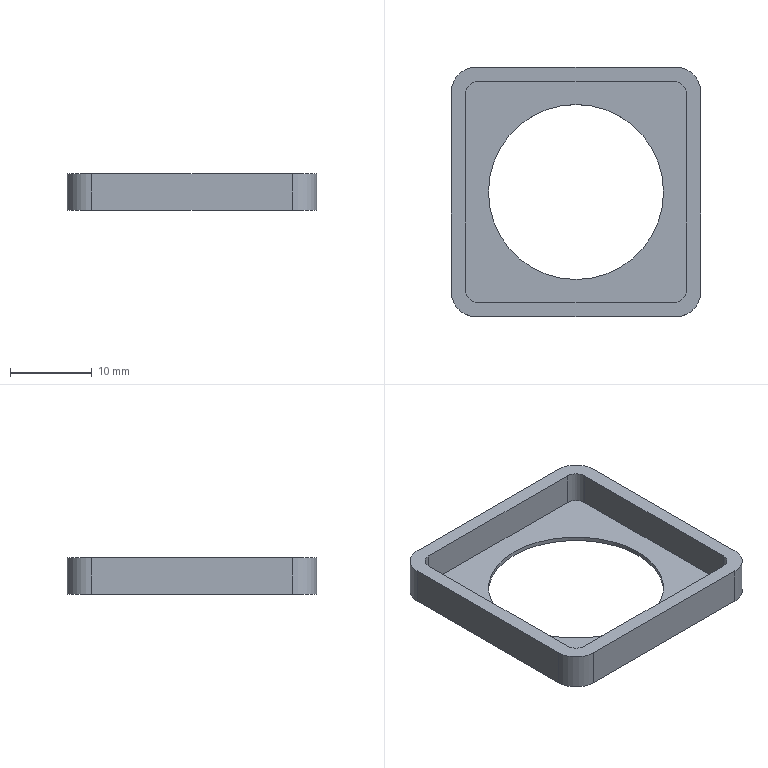Part | STEP file | 1 solid | 21 faces | box 30.5 x 30.5 x 4.5 mm | volume 1063 mm3 | plane 11 | cylinder 10 | commonest cylinder face diameters 3 x4 6 x4 21.4 x2
STEP:
#1=CARTESIAN_POINT('',(10.7,0.,0.));
#2=VERTEX_POINT('',#1);
#3=CARTESIAN_POINT('',(-10.7,0.,0.));
#4=VERTEX_POINT('',#3);
#5=CARTESIAN_POINT('',(0.,0.,0.));
#6=DIRECTION('',(0.,0.,-1.));
#7=DIRECTION('',(-1.,0.,0.));
#8=AXIS2_PLACEMENT_3D('',#5,#6,#7);
#9=CIRCLE('',#8,10.7);
#10=EDGE_CURVE('',#2,#4,#9,.T.);
#11=ORIENTED_EDGE('',*,*,#10,.T.);
#12=CARTESIAN_POINT('',(-10.7,0.,0.5));
#13=VERTEX_POINT('',#12);
#14=CARTESIAN_POINT('',(-10.7,0.,-3.4));
#15=DIRECTION('',(0.,0.,1.));
#16=VECTOR('',#15,1000.);
#17=LINE('',#14,#16);
#18=EDGE_CURVE('',#4,#13,#17,.T.);
#19=ORIENTED_EDGE('',*,*,#18,.T.);
#20=CARTESIAN_POINT('',(10.7,0.,0.5));
#21=VERTEX_POINT('',#20);
#22=CARTESIAN_POINT('',(0.,0.,0.5));
#23=DIRECTION('',(0.,0.,1.));
#24=DIRECTION('',(1.,0.,0.));
#25=AXIS2_PLACEMENT_3D('',#22,#23,#24);
#26=CIRCLE('',#25,10.7);
#27=EDGE_CURVE('',#13,#21,#26,.T.);
#28=ORIENTED_EDGE('',*,*,#27,.T.);
#29=CARTESIAN_POINT('',(10.7,0.,-3.4));
#30=DIRECTION('',(0.,0.,1.));
#31=VECTOR('',#30,1000.);
#32=LINE('',#29,#31);
#33=EDGE_CURVE('',#2,#21,#32,.T.);
#34=ORIENTED_EDGE('',*,*,#33,.F.);
#35=EDGE_LOOP('',(#11,#19,#28,#34));
#36=FACE_OUTER_BOUND('',#35,.T.);
#37=CARTESIAN_POINT('',(0.,0.,-3.4));
#38=DIRECTION('',(0.,0.,1.));
#39=DIRECTION('',(1.,0.,0.));
#40=AXIS2_PLACEMENT_3D('',#37,#38,#39);
#41=CYLINDRICAL_SURFACE('',#40,10.7);
#42=ADVANCED_FACE('',(#36),#41,.F.);
#43=CARTESIAN_POINT('',(-15.25,-12.25,0.));
#44=VERTEX_POINT('',#43);
#45=CARTESIAN_POINT('',(-12.25,-15.25,0.));
#46=VERTEX_POINT('',#45);
#47=CARTESIAN_POINT('',(-12.25,-12.25,0.));
#48=DIRECTION('',(0.,0.,1.));
#49=DIRECTION('',(-1.,0.,0.));
#50=AXIS2_PLACEMENT_3D('',#47,#48,#49);
#51=CIRCLE('',#50,3.);
#52=EDGE_CURVE('',#44,#46,#51,.T.);
#53=ORIENTED_EDGE('',*,*,#52,.T.);
#54=CARTESIAN_POINT('',(-12.25,-15.25,4.5));
#55=VERTEX_POINT('',#54);
#56=CARTESIAN_POINT('',(-12.25,-15.25,4.5));
#57=DIRECTION('',(0.,0.,-1.));
#58=VECTOR('',#57,1000.);
#59=LINE('',#56,#58);
#60=EDGE_CURVE('',#55,#46,#59,.T.);
#61=ORIENTED_EDGE('',*,*,#60,.F.);
#62=CARTESIAN_POINT('',(-15.25,-12.25,4.5));
#63=VERTEX_POINT('',#62);
#64=CARTESIAN_POINT('',(-12.25,-12.25,4.5));
#65=DIRECTION('',(0.,0.,1.));
#66=DIRECTION('',(-1.,0.,0.));
#67=AXIS2_PLACEMENT_3D('',#64,#65,#66);
#68=CIRCLE('',#67,3.);
#69=EDGE_CURVE('',#63,#55,#68,.T.);
#70=ORIENTED_EDGE('',*,*,#69,.F.);
#71=CARTESIAN_POINT('',(-15.25,-12.25,4.5));
#72=DIRECTION('',(0.,0.,-1.));
#73=VECTOR('',#72,1000.);
#74=LINE('',#71,#73);
#75=EDGE_CURVE('',#63,#44,#74,.T.);
#76=ORIENTED_EDGE('',*,*,#75,.T.);
#77=EDGE_LOOP('',(#53,#61,#70,#76));
#78=FACE_OUTER_BOUND('',#77,.T.);
#79=CARTESIAN_POINT('',(-12.25,-12.25,4.5));
#80=DIRECTION('',(0.,0.,-1.));
#81=DIRECTION('',(-1.,0.,0.));
#82=AXIS2_PLACEMENT_3D('',#79,#80,#81);
#83=CYLINDRICAL_SURFACE('',#82,3.);
#84=ADVANCED_FACE('',(#78),#83,.T.);
#85=CARTESIAN_POINT('',(12.25,-15.25,0.));
#86=VERTEX_POINT('',#85);
#87=CARTESIAN_POINT('',(-12.25,-15.25,0.));
#88=DIRECTION('',(1.,0.,0.));
#89=VECTOR('',#88,1000.);
#90=LINE('',#87,#89);
#91=EDGE_CURVE('',#46,#86,#90,.T.);
#92=ORIENTED_EDGE('',*,*,#91,.T.);
#93=CARTESIAN_POINT('',(12.25,-15.25,4.5));
#94=VERTEX_POINT('',#93);
#95=CARTESIAN_POINT('',(12.25,-15.25,4.5));
#96=DIRECTION('',(0.,0.,-1.));
#97=VECTOR('',#96,1000.);
#98=LINE('',#95,#97);
#99=EDGE_CURVE('',#94,#86,#98,.T.);
#100=ORIENTED_EDGE('',*,*,#99,.F.);
#101=CARTESIAN_POINT('',(-12.25,-15.25,4.5));
#102=DIRECTION('',(1.,0.,0.));
#103=VECTOR('',#102,1000.);
#104=LINE('',#101,#103);
#105=EDGE_CURVE('',#55,#94,#104,.T.);
#106=ORIENTED_EDGE('',*,*,#105,.F.);
#107=ORIENTED_EDGE('',*,*,#60,.T.);
#108=EDGE_LOOP('',(#92,#100,#106,#107));
#109=FACE_OUTER_BOUND('',#108,.T.);
#110=CARTESIAN_POINT('',(-12.25,-15.25,4.5));
#111=DIRECTION('',(0.,1.,0.));
#112=DIRECTION('',(1.,0.,0.));
#113=AXIS2_PLACEMENT_3D('',#110,#111,#112);
#114=PLANE('',#113);
#115=ADVANCED_FACE('',(#109),#114,.F.);
#116=CARTESIAN_POINT('',(15.25,-12.25,0.));
#117=VERTEX_POINT('',#116);
#118=CARTESIAN_POINT('',(12.25,-12.25,0.));
#119=DIRECTION('',(0.,0.,1.));
#120=DIRECTION('',(1.,0.,0.));
#121=AXIS2_PLACEMENT_3D('',#118,#119,#120);
#122=CIRCLE('',#121,3.);
#123=EDGE_CURVE('',#86,#117,#122,.T.);
#124=ORIENTED_EDGE('',*,*,#123,.T.);
#125=CARTESIAN_POINT('',(15.25,-12.25,4.5));
#126=VERTEX_POINT('',#125);
#127=CARTESIAN_POINT('',(15.25,-12.25,4.5));
#128=DIRECTION('',(0.,0.,-1.));
#129=VECTOR('',#128,1000.);
#130=LINE('',#127,#129);
#131=EDGE_CURVE('',#126,#117,#130,.T.);
#132=ORIENTED_EDGE('',*,*,#131,.F.);
#133=CARTESIAN_POINT('',(12.25,-12.25,4.5));
#134=DIRECTION('',(0.,0.,1.));
#135=DIRECTION('',(1.,0.,0.));
#136=AXIS2_PLACEMENT_3D('',#133,#134,#135);
#137=CIRCLE('',#136,3.);
#138=EDGE_CURVE('',#94,#126,#137,.T.);
#139=ORIENTED_EDGE('',*,*,#138,.F.);
#140=ORIENTED_EDGE('',*,*,#99,.T.);
#141=EDGE_LOOP('',(#124,#132,#139,#140));
#142=FACE_OUTER_BOUND('',#141,.T.);
#143=CARTESIAN_POINT('',(12.25,-12.25,4.5));
#144=DIRECTION('',(0.,0.,-1.));
#145=DIRECTION('',(-1.,0.,0.));
#146=AXIS2_PLACEMENT_3D('',#143,#144,#145);
#147=CYLINDRICAL_SURFACE('',#146,3.);
#148=ADVANCED_FACE('',(#142),#147,.T.);
#149=CARTESIAN_POINT('',(15.25,12.25,0.));
#150=VERTEX_POINT('',#149);
#151=CARTESIAN_POINT('',(15.25,-12.25,0.));
#152=DIRECTION('',(0.,1.,0.));
#153=VECTOR('',#152,1000.);
#154=LINE('',#151,#153);
#155=EDGE_CURVE('',#117,#150,#154,.T.);
#156=ORIENTED_EDGE('',*,*,#155,.T.);
#157=CARTESIAN_POINT('',(15.25,12.25,4.5));
#158=VERTEX_POINT('',#157);
#159=CARTESIAN_POINT('',(15.25,12.25,4.5));
#160=DIRECTION('',(0.,0.,-1.));
#161=VECTOR('',#160,1000.);
#162=LINE('',#159,#161);
#163=EDGE_CURVE('',#158,#150,#162,.T.);
#164=ORIENTED_EDGE('',*,*,#163,.F.);
#165=CARTESIAN_POINT('',(15.25,-12.25,4.5));
#166=DIRECTION('',(0.,1.,0.));
#167=VECTOR('',#166,1000.);
#168=LINE('',#165,#167);
#169=EDGE_CURVE('',#126,#158,#168,.T.);
#170=ORIENTED_EDGE('',*,*,#169,.F.);
#171=ORIENTED_EDGE('',*,*,#131,.T.);
#172=EDGE_LOOP('',(#156,#164,#170,#171));
#173=FACE_OUTER_BOUND('',#172,.T.);
#174=CARTESIAN_POINT('',(15.25,-12.25,4.5));
#175=DIRECTION('',(-1.,0.,0.));
#176=DIRECTION('',(0.,0.,1.));
#177=AXIS2_PLACEMENT_3D('',#174,#175,#176);
#178=PLANE('',#177);
#179=ADVANCED_FACE('',(#173),#178,.F.);
#180=CARTESIAN_POINT('',(12.25,15.25,0.));
#181=VERTEX_POINT('',#180);
#182=CARTESIAN_POINT('',(12.25,12.25,0.));
#183=DIRECTION('',(0.,0.,1.));
#184=DIRECTION('',(-1.,0.,0.));
#185=AXIS2_PLACEMENT_3D('',#182,#183,#184);
#186=CIRCLE('',#185,3.);
#187=EDGE_CURVE('',#150,#181,#186,.T.);
#188=ORIENTED_EDGE('',*,*,#187,.T.);
#189=CARTESIAN_POINT('',(12.25,15.25,4.5));
#190=VERTEX_POINT('',#189);
#191=CARTESIAN_POINT('',(12.25,15.25,4.5));
#192=DIRECTION('',(0.,0.,-1.));
#193=VECTOR('',#192,1000.);
#194=LINE('',#191,#193);
#195=EDGE_CURVE('',#190,#181,#194,.T.);
#196=ORIENTED_EDGE('',*,*,#195,.F.);
#197=CARTESIAN_POINT('',(12.25,12.25,4.5));
#198=DIRECTION('',(0.,0.,1.));
#199=DIRECTION('',(-1.,0.,0.));
#200=AXIS2_PLACEMENT_3D('',#197,#198,#199);
#201=CIRCLE('',#200,3.);
#202=EDGE_CURVE('',#158,#190,#201,.T.);
#203=ORIENTED_EDGE('',*,*,#202,.F.);
#204=ORIENTED_EDGE('',*,*,#163,.T.);
#205=EDGE_LOOP('',(#188,#196,#203,#204));
#206=FACE_OUTER_BOUND('',#205,.T.);
#207=CARTESIAN_POINT('',(12.25,12.25,4.5));
#208=DIRECTION('',(0.,0.,-1.));
#209=DIRECTION('',(-1.,0.,0.));
#210=AXIS2_PLACEMENT_3D('',#207,#208,#209);
#211=CYLINDRICAL_SURFACE('',#210,3.);
#212=ADVANCED_FACE('',(#206),#211,.T.);
#213=CARTESIAN_POINT('',(-12.25,15.25,0.));
#214=VERTEX_POINT('',#213);
#215=CARTESIAN_POINT('',(-12.25,15.25,0.));
#216=DIRECTION('',(-1.,0.,0.));
#217=VECTOR('',#216,1000.);
#218=LINE('',#215,#217);
#219=EDGE_CURVE('',#181,#214,#218,.T.);
#220=ORIENTED_EDGE('',*,*,#219,.T.);
#221=CARTESIAN_POINT('',(-12.25,15.25,4.5));
#222=VERTEX_POINT('',#221);
#223=CARTESIAN_POINT('',(-12.25,15.25,4.5));
#224=DIRECTION('',(0.,0.,-1.));
#225=VECTOR('',#224,1000.);
#226=LINE('',#223,#225);
#227=EDGE_CURVE('',#222,#214,#226,.T.);
#228=ORIENTED_EDGE('',*,*,#227,.F.);
#229=CARTESIAN_POINT('',(-12.25,15.25,4.5));
#230=DIRECTION('',(-1.,0.,0.));
#231=VECTOR('',#230,1000.);
#232=LINE('',#229,#231);
#233=EDGE_CURVE('',#190,#222,#232,.T.);
#234=ORIENTED_EDGE('',*,*,#233,.F.);
#235=ORIENTED_EDGE('',*,*,#195,.T.);
#236=EDGE_LOOP('',(#220,#228,#234,#235));
#237=FACE_OUTER_BOUND('',#236,.T.);
#238=CARTESIAN_POINT('',(-12.25,15.25,4.5));
#239=DIRECTION('',(0.,-1.,0.));
#240=DIRECTION('',(0.,0.,-1.));
#241=AXIS2_PLACEMENT_3D('',#238,#239,#240);
#242=PLANE('',#241);
#243=ADVANCED_FACE('',(#237),#242,.F.);
#244=CARTESIAN_POINT('',(-15.25,12.25,0.));
#245=VERTEX_POINT('',#244);
#246=CARTESIAN_POINT('',(-12.25,12.25,0.));
#247=DIRECTION('',(0.,0.,1.));
#248=DIRECTION('',(-1.,0.,0.));
#249=AXIS2_PLACEMENT_3D('',#246,#247,#248);
#250=CIRCLE('',#249,3.);
#251=EDGE_CURVE('',#214,#245,#250,.T.);
#252=ORIENTED_EDGE('',*,*,#251,.T.);
#253=CARTESIAN_POINT('',(-15.25,12.25,4.5));
#254=VERTEX_POINT('',#253);
#255=CARTESIAN_POINT('',(-15.25,12.25,4.5));
#256=DIRECTION('',(0.,0.,-1.));
#257=VECTOR('',#256,1000.);
#258=LINE('',#255,#257);
#259=EDGE_CURVE('',#254,#245,#258,.T.);
#260=ORIENTED_EDGE('',*,*,#259,.F.);
#261=CARTESIAN_POINT('',(-12.25,12.25,4.5));
#262=DIRECTION('',(0.,0.,1.));
#263=DIRECTION('',(-1.,0.,0.));
#264=AXIS2_PLACEMENT_3D('',#261,#262,#263);
#265=CIRCLE('',#264,3.);
#266=EDGE_CURVE('',#222,#254,#265,.T.);
#267=ORIENTED_EDGE('',*,*,#266,.F.);
#268=ORIENTED_EDGE('',*,*,#227,.T.);
#269=EDGE_LOOP('',(#252,#260,#267,#268));
#270=FACE_OUTER_BOUND('',#269,.T.);
#271=CARTESIAN_POINT('',(-12.25,12.25,4.5));
#272=DIRECTION('',(0.,0.,-1.));
#273=DIRECTION('',(-1.,0.,0.));
#274=AXIS2_PLACEMENT_3D('',#271,#272,#273);
#275=CYLINDRICAL_SURFACE('',#274,3.);
#276=ADVANCED_FACE('',(#270),#275,.T.);
#277=CARTESIAN_POINT('',(-15.25,-12.25,0.));
#278=DIRECTION('',(0.,-1.,0.));
#279=VECTOR('',#278,1000.);
#280=LINE('',#277,#279);
#281=EDGE_CURVE('',#245,#44,#280,.T.);
#282=ORIENTED_EDGE('',*,*,#281,.T.);
#283=ORIENTED_EDGE('',*,*,#75,.F.);
#284=CARTESIAN_POINT('',(-15.25,-12.25,4.5));
#285=DIRECTION('',(0.,-1.,0.));
#286=VECTOR('',#285,1000.);
#287=LINE('',#284,#286);
#288=EDGE_CURVE('',#254,#63,#287,.T.);
#289=ORIENTED_EDGE('',*,*,#288,.F.);
#290=ORIENTED_EDGE('',*,*,#259,.T.);
#291=EDGE_LOOP('',(#282,#283,#289,#290));
#292=FACE_OUTER_BOUND('',#291,.T.);
#293=CARTESIAN_POINT('',(-15.25,-12.25,4.5));
#294=DIRECTION('',(1.,0.,0.));
#295=DIRECTION('',(0.,1.,0.));
#296=AXIS2_PLACEMENT_3D('',#293,#294,#295);
#297=PLANE('',#296);
#298=ADVANCED_FACE('',(#292),#297,.F.);
#299=ORIENTED_EDGE('',*,*,#69,.T.);
#300=ORIENTED_EDGE('',*,*,#105,.T.);
#301=ORIENTED_EDGE('',*,*,#138,.T.);
#302=ORIENTED_EDGE('',*,*,#169,.T.);
#303=ORIENTED_EDGE('',*,*,#202,.T.);
#304=ORIENTED_EDGE('',*,*,#233,.T.);
#305=ORIENTED_EDGE('',*,*,#266,.T.);
#306=ORIENTED_EDGE('',*,*,#288,.T.);
#307=EDGE_LOOP('',(#299,#300,#301,#302,#303,#304,#305,#306));
#308=FACE_OUTER_BOUND('',#307,.T.);
#309=CARTESIAN_POINT('',(-12.,-13.5,4.5));
#310=VERTEX_POINT('',#309);
#311=CARTESIAN_POINT('',(12.,-13.5,4.5));
#312=VERTEX_POINT('',#311);
#313=CARTESIAN_POINT('',(-12.,-13.5,4.5));
#314=DIRECTION('',(1.,0.,0.));
#315=VECTOR('',#314,1000.);
#316=LINE('',#313,#315);
#317=EDGE_CURVE('',#310,#312,#316,.T.);
#318=ORIENTED_EDGE('',*,*,#317,.F.);
#319=CARTESIAN_POINT('',(-13.5,-12.,4.5));
#320=VERTEX_POINT('',#319);
#321=CARTESIAN_POINT('',(-12.,-12.,4.5));
#322=DIRECTION('',(0.,0.,1.));
#323=DIRECTION('',(-1.,0.,0.));
#324=AXIS2_PLACEMENT_3D('',#321,#322,#323);
#325=CIRCLE('',#324,1.5);
#326=EDGE_CURVE('',#320,#310,#325,.T.);
#327=ORIENTED_EDGE('',*,*,#326,.F.);
#328=CARTESIAN_POINT('',(-13.5,12.,4.5));
#329=VERTEX_POINT('',#328);
#330=CARTESIAN_POINT('',(-13.5,-12.,4.5));
#331=DIRECTION('',(0.,-1.,0.));
#332=VECTOR('',#331,1000.);
#333=LINE('',#330,#332);
#334=EDGE_CURVE('',#329,#320,#333,.T.);
#335=ORIENTED_EDGE('',*,*,#334,.F.);
#336=CARTESIAN_POINT('',(-12.,13.5,4.5));
#337=VERTEX_POINT('',#336);
#338=CARTESIAN_POINT('',(-12.,12.,4.5));
#339=DIRECTION('',(0.,0.,1.));
#340=DIRECTION('',(-1.,0.,0.));
#341=AXIS2_PLACEMENT_3D('',#338,#339,#340);
#342=CIRCLE('',#341,1.5);
#343=EDGE_CURVE('',#337,#329,#342,.T.);
#344=ORIENTED_EDGE('',*,*,#343,.F.);
#345=CARTESIAN_POINT('',(12.,13.5,4.5));
#346=VERTEX_POINT('',#345);
#347=CARTESIAN_POINT('',(-12.,13.5,4.5));
#348=DIRECTION('',(-1.,0.,0.));
#349=VECTOR('',#348,1000.);
#350=LINE('',#347,#349);
#351=EDGE_CURVE('',#346,#337,#350,.T.);
#352=ORIENTED_EDGE('',*,*,#351,.F.);
#353=CARTESIAN_POINT('',(13.5,12.,4.5));
#354=VERTEX_POINT('',#353);
#355=CARTESIAN_POINT('',(12.,12.,4.5));
#356=DIRECTION('',(0.,0.,1.));
#357=DIRECTION('',(-1.,0.,0.));
#358=AXIS2_PLACEMENT_3D('',#355,#356,#357);
#359=CIRCLE('',#358,1.5);
#360=EDGE_CURVE('',#354,#346,#359,.T.);
#361=ORIENTED_EDGE('',*,*,#360,.F.);
#362=CARTESIAN_POINT('',(13.5,-12.,4.5));
#363=VERTEX_POINT('',#362);
#364=CARTESIAN_POINT('',(13.5,-12.,4.5));
#365=DIRECTION('',(0.,1.,0.));
#366=VECTOR('',#365,1000.);
#367=LINE('',#364,#366);
#368=EDGE_CURVE('',#363,#354,#367,.T.);
#369=ORIENTED_EDGE('',*,*,#368,.F.);
#370=CARTESIAN_POINT('',(12.,-12.,4.5));
#371=DIRECTION('',(0.,0.,1.));
#372=DIRECTION('',(1.,0.,0.));
#373=AXIS2_PLACEMENT_3D('',#370,#371,#372);
#374=CIRCLE('',#373,1.5);
#375=EDGE_CURVE('',#312,#363,#374,.T.);
#376=ORIENTED_EDGE('',*,*,#375,.F.);
#377=EDGE_LOOP('',(#318,#327,#335,#344,#352,#361,#369,#376));
#378=FACE_BOUND('',#377,.T.);
#379=CARTESIAN_POINT('',(-12.25,-12.25,4.5));
#380=DIRECTION('',(0.,0.,-1.));
#381=DIRECTION('',(0.,-1.,0.));
#382=AXIS2_PLACEMENT_3D('',#379,#380,#381);
#383=PLANE('',#382);
#384=ADVANCED_FACE('',(#308,#378),#383,.F.);
#385=ORIENTED_EDGE('',*,*,#52,.F.);
#386=ORIENTED_EDGE('',*,*,#281,.F.);
#387=ORIENTED_EDGE('',*,*,#251,.F.);
#388=ORIENTED_EDGE('',*,*,#219,.F.);
#389=ORIENTED_EDGE('',*,*,#187,.F.);
#390=ORIENTED_EDGE('',*,*,#155,.F.);
#391=ORIENTED_EDGE('',*,*,#123,.F.);
#392=ORIENTED_EDGE('',*,*,#91,.F.);
#393=EDGE_LOOP('',(#385,#386,#387,#388,#389,#390,#391,#392));
#394=FACE_OUTER_BOUND('',#393,.T.);
#395=ORIENTED_EDGE('',*,*,#10,.F.);
#396=CARTESIAN_POINT('',(0.,0.,0.));
#397=DIRECTION('',(0.,0.,-1.));
#398=DIRECTION('',(-1.,0.,0.));
#399=AXIS2_PLACEMENT_3D('',#396,#397,#398);
#400=CIRCLE('',#399,10.7);
#401=EDGE_CURVE('',#4,#2,#400,.T.);
#402=ORIENTED_EDGE('',*,*,#401,.F.);
#403=EDGE_LOOP('',(#395,#402));
#404=FACE_BOUND('',#403,.T.);
#405=CARTESIAN_POINT('',(-12.25,-12.25,0.));
#406=DIRECTION('',(0.,0.,-1.));
#407=DIRECTION('',(0.,-1.,0.));
#408=AXIS2_PLACEMENT_3D('',#405,#406,#407);
#409=PLANE('',#408);
#410=ADVANCED_FACE('',(#394,#404),#409,.T.);
#411=ORIENTED_EDGE('',*,*,#326,.T.);
#412=CARTESIAN_POINT('',(-12.,-13.5,0.5));
#413=VERTEX_POINT('',#412);
#414=CARTESIAN_POINT('',(-12.,-13.5,0.5));
#415=DIRECTION('',(0.,0.,1.));
#416=VECTOR('',#415,1000.);
#417=LINE('',#414,#416);
#418=EDGE_CURVE('',#413,#310,#417,.T.);
#419=ORIENTED_EDGE('',*,*,#418,.F.);
#420=CARTESIAN_POINT('',(-13.5,-12.,0.5));
#421=VERTEX_POINT('',#420);
#422=CARTESIAN_POINT('',(-12.,-12.,0.5));
#423=DIRECTION('',(0.,0.,1.));
#424=DIRECTION('',(-1.,0.,0.));
#425=AXIS2_PLACEMENT_3D('',#422,#423,#424);
#426=CIRCLE('',#425,1.5);
#427=EDGE_CURVE('',#421,#413,#426,.T.);
#428=ORIENTED_EDGE('',*,*,#427,.F.);
#429=CARTESIAN_POINT('',(-13.5,-12.,0.5));
#430=DIRECTION('',(0.,0.,1.));
#431=VECTOR('',#430,1000.);
#432=LINE('',#429,#431);
#433=EDGE_CURVE('',#421,#320,#432,.T.);
#434=ORIENTED_EDGE('',*,*,#433,.T.);
#435=EDGE_LOOP('',(#411,#419,#428,#434));
#436=FACE_OUTER_BOUND('',#435,.T.);
#437=CARTESIAN_POINT('',(-12.,-12.,0.5));
#438=DIRECTION('',(0.,0.,1.));
#439=DIRECTION('',(1.,0.,0.));
#440=AXIS2_PLACEMENT_3D('',#437,#438,#439);
#441=CYLINDRICAL_SURFACE('',#440,1.5);
#442=ADVANCED_FACE('',(#436),#441,.F.);
#443=ORIENTED_EDGE('',*,*,#334,.T.);
#444=ORIENTED_EDGE('',*,*,#433,.F.);
#445=CARTESIAN_POINT('',(-13.5,12.,0.5));
#446=VERTEX_POINT('',#445);
#447=CARTESIAN_POINT('',(-13.5,-12.,0.5));
#448=DIRECTION('',(0.,-1.,0.));
#449=VECTOR('',#448,1000.);
#450=LINE('',#447,#449);
#451=EDGE_CURVE('',#446,#421,#450,.T.);
#452=ORIENTED_EDGE('',*,*,#451,.F.);
#453=CARTESIAN_POINT('',(-13.5,12.,0.5));
#454=DIRECTION('',(0.,0.,1.));
#455=VECTOR('',#454,1000.);
#456=LINE('',#453,#455);
#457=EDGE_CURVE('',#446,#329,#456,.T.);
#458=ORIENTED_EDGE('',*,*,#457,.T.);
#459=EDGE_LOOP('',(#443,#444,#452,#458));
#460=FACE_OUTER_BOUND('',#459,.T.);
#461=CARTESIAN_POINT('',(-13.5,-12.,0.5));
#462=DIRECTION('',(-1.,0.,0.));
#463=DIRECTION('',(0.,0.,1.));
#464=AXIS2_PLACEMENT_3D('',#461,#462,#463);
#465=PLANE('',#464);
#466=ADVANCED_FACE('',(#460),#465,.F.);
#467=ORIENTED_EDGE('',*,*,#343,.T.);
#468=ORIENTED_EDGE('',*,*,#457,.F.);
#469=CARTESIAN_POINT('',(-12.,13.5,0.5));
#470=VERTEX_POINT('',#469);
#471=CARTESIAN_POINT('',(-12.,12.,0.5));
#472=DIRECTION('',(0.,0.,1.));
#473=DIRECTION('',(-1.,0.,0.));
#474=AXIS2_PLACEMENT_3D('',#471,#472,#473);
#475=CIRCLE('',#474,1.5);
#476=EDGE_CURVE('',#470,#446,#475,.T.);
#477=ORIENTED_EDGE('',*,*,#476,.F.);
#478=CARTESIAN_POINT('',(-12.,13.5,0.5));
#479=DIRECTION('',(0.,0.,1.));
#480=VECTOR('',#479,1000.);
#481=LINE('',#478,#480);
#482=EDGE_CURVE('',#470,#337,#481,.T.);
#483=ORIENTED_EDGE('',*,*,#482,.T.);
#484=EDGE_LOOP('',(#467,#468,#477,#483));
#485=FACE_OUTER_BOUND('',#484,.T.);
#486=CARTESIAN_POINT('',(-12.,12.,0.5));
#487=DIRECTION('',(0.,0.,1.));
#488=DIRECTION('',(1.,0.,0.));
#489=AXIS2_PLACEMENT_3D('',#486,#487,#488);
#490=CYLINDRICAL_SURFACE('',#489,1.5);
#491=ADVANCED_FACE('',(#485),#490,.F.);
#492=ORIENTED_EDGE('',*,*,#351,.T.);
#493=ORIENTED_EDGE('',*,*,#482,.F.);
#494=CARTESIAN_POINT('',(12.,13.5,0.5));
#495=VERTEX_POINT('',#494);
#496=CARTESIAN_POINT('',(-12.,13.5,0.5));
#497=DIRECTION('',(-1.,0.,0.));
#498=VECTOR('',#497,1000.);
#499=LINE('',#496,#498);
#500=EDGE_CURVE('',#495,#470,#499,.T.);
#501=ORIENTED_EDGE('',*,*,#500,.F.);
#502=CARTESIAN_POINT('',(12.,13.5,0.5));
#503=DIRECTION('',(0.,0.,1.));
#504=VECTOR('',#503,1000.);
#505=LINE('',#502,#504);
#506=EDGE_CURVE('',#495,#346,#505,.T.);
#507=ORIENTED_EDGE('',*,*,#506,.T.);
#508=EDGE_LOOP('',(#492,#493,#501,#507));
#509=FACE_OUTER_BOUND('',#508,.T.);
#510=CARTESIAN_POINT('',(-12.,13.5,0.5));
#511=DIRECTION('',(0.,1.,0.));
#512=DIRECTION('',(1.,0.,0.));
#513=AXIS2_PLACEMENT_3D('',#510,#511,#512);
#514=PLANE('',#513);
#515=ADVANCED_FACE('',(#509),#514,.F.);
#516=ORIENTED_EDGE('',*,*,#360,.T.);
#517=ORIENTED_EDGE('',*,*,#506,.F.);
#518=CARTESIAN_POINT('',(13.5,12.,0.5));
#519=VERTEX_POINT('',#518);
#520=CARTESIAN_POINT('',(12.,12.,0.5));
#521=DIRECTION('',(0.,0.,1.));
#522=DIRECTION('',(-1.,0.,0.));
#523=AXIS2_PLACEMENT_3D('',#520,#521,#522);
#524=CIRCLE('',#523,1.5);
#525=EDGE_CURVE('',#519,#495,#524,.T.);
#526=ORIENTED_EDGE('',*,*,#525,.F.);
#527=CARTESIAN_POINT('',(13.5,12.,0.5));
#528=DIRECTION('',(0.,0.,1.));
#529=VECTOR('',#528,1000.);
#530=LINE('',#527,#529);
#531=EDGE_CURVE('',#519,#354,#530,.T.);
#532=ORIENTED_EDGE('',*,*,#531,.T.);
#533=EDGE_LOOP('',(#516,#517,#526,#532));
#534=FACE_OUTER_BOUND('',#533,.T.);
#535=CARTESIAN_POINT('',(12.,12.,0.5));
#536=DIRECTION('',(0.,0.,1.));
#537=DIRECTION('',(1.,0.,0.));
#538=AXIS2_PLACEMENT_3D('',#535,#536,#537);
#539=CYLINDRICAL_SURFACE('',#538,1.5);
#540=ADVANCED_FACE('',(#534),#539,.F.);
#541=ORIENTED_EDGE('',*,*,#368,.T.);
#542=ORIENTED_EDGE('',*,*,#531,.F.);
#543=CARTESIAN_POINT('',(13.5,-12.,0.5));
#544=VERTEX_POINT('',#543);
#545=CARTESIAN_POINT('',(13.5,-12.,0.5));
#546=DIRECTION('',(0.,1.,0.));
#547=VECTOR('',#546,1000.);
#548=LINE('',#545,#547);
#549=EDGE_CURVE('',#544,#519,#548,.T.);
#550=ORIENTED_EDGE('',*,*,#549,.F.);
#551=CARTESIAN_POINT('',(13.5,-12.,0.5));
#552=DIRECTION('',(0.,0.,1.));
#553=VECTOR('',#552,1000.);
#554=LINE('',#551,#553);
#555=EDGE_CURVE('',#544,#363,#554,.T.);
#556=ORIENTED_EDGE('',*,*,#555,.T.);
#557=EDGE_LOOP('',(#541,#542,#550,#556));
#558=FACE_OUTER_BOUND('',#557,.T.);
#559=CARTESIAN_POINT('',(13.5,-12.,0.5));
#560=DIRECTION('',(1.,0.,0.));
#561=DIRECTION('',(0.,1.,0.));
#562=AXIS2_PLACEMENT_3D('',#559,#560,#561);
#563=PLANE('',#562);
#564=ADVANCED_FACE('',(#558),#563,.F.);
#565=ORIENTED_EDGE('',*,*,#375,.T.);
#566=ORIENTED_EDGE('',*,*,#555,.F.);
#567=CARTESIAN_POINT('',(12.,-13.5,0.5));
#568=VERTEX_POINT('',#567);
#569=CARTESIAN_POINT('',(12.,-12.,0.5));
#570=DIRECTION('',(0.,0.,1.));
#571=DIRECTION('',(1.,0.,0.));
#572=AXIS2_PLACEMENT_3D('',#569,#570,#571);
#573=CIRCLE('',#572,1.5);
#574=EDGE_CURVE('',#568,#544,#573,.T.);
#575=ORIENTED_EDGE('',*,*,#574,.F.);
#576=CARTESIAN_POINT('',(12.,-13.5,0.5));
#577=DIRECTION('',(0.,0.,1.));
#578=VECTOR('',#577,1000.);
#579=LINE('',#576,#578);
#580=EDGE_CURVE('',#568,#312,#579,.T.);
#581=ORIENTED_EDGE('',*,*,#580,.T.);
#582=EDGE_LOOP('',(#565,#566,#575,#581));
#583=FACE_OUTER_BOUND('',#582,.T.);
#584=CARTESIAN_POINT('',(12.,-12.,0.5));
#585=DIRECTION('',(0.,0.,1.));
#586=DIRECTION('',(1.,0.,0.));
#587=AXIS2_PLACEMENT_3D('',#584,#585,#586);
#588=CYLINDRICAL_SURFACE('',#587,1.5);
#589=ADVANCED_FACE('',(#583),#588,.F.);
#590=ORIENTED_EDGE('',*,*,#317,.T.);
#591=ORIENTED_EDGE('',*,*,#580,.F.);
#592=CARTESIAN_POINT('',(-12.,-13.5,0.5));
#593=DIRECTION('',(1.,0.,0.));
#594=VECTOR('',#593,1000.);
#595=LINE('',#592,#594);
#596=EDGE_CURVE('',#413,#568,#595,.T.);
#597=ORIENTED_EDGE('',*,*,#596,.F.);
#598=ORIENTED_EDGE('',*,*,#418,.T.);
#599=EDGE_LOOP('',(#590,#591,#597,#598));
#600=FACE_OUTER_BOUND('',#599,.T.);
#601=CARTESIAN_POINT('',(-12.,-13.5,0.5));
#602=DIRECTION('',(0.,-1.,0.));
#603=DIRECTION('',(0.,0.,-1.));
#604=AXIS2_PLACEMENT_3D('',#601,#602,#603);
#605=PLANE('',#604);
#606=ADVANCED_FACE('',(#600),#605,.F.);
#607=ORIENTED_EDGE('',*,*,#427,.T.);
#608=ORIENTED_EDGE('',*,*,#596,.T.);
#609=ORIENTED_EDGE('',*,*,#574,.T.);
#610=ORIENTED_EDGE('',*,*,#549,.T.);
#611=ORIENTED_EDGE('',*,*,#525,.T.);
#612=ORIENTED_EDGE('',*,*,#500,.T.);
#613=ORIENTED_EDGE('',*,*,#476,.T.);
#614=ORIENTED_EDGE('',*,*,#451,.T.);
#615=EDGE_LOOP('',(#607,#608,#609,#610,#611,#612,#613,#614));
#616=FACE_OUTER_BOUND('',#615,.T.);
#617=CARTESIAN_POINT('',(0.,0.,0.5));
#618=DIRECTION('',(0.,0.,1.));
#619=DIRECTION('',(1.,0.,0.));
#620=AXIS2_PLACEMENT_3D('',#617,#618,#619);
#621=CIRCLE('',#620,10.7);
#622=EDGE_CURVE('',#21,#13,#621,.T.);
#623=ORIENTED_EDGE('',*,*,#622,.F.);
#624=ORIENTED_EDGE('',*,*,#27,.F.);
#625=EDGE_LOOP('',(#623,#624));
#626=FACE_BOUND('',#625,.T.);
#627=CARTESIAN_POINT('',(-12.,-12.,0.5));
#628=DIRECTION('',(0.,0.,-1.));
#629=DIRECTION('',(0.,-1.,0.));
#630=AXIS2_PLACEMENT_3D('',#627,#628,#629);
#631=PLANE('',#630);
#632=ADVANCED_FACE('',(#616,#626),#631,.F.);
#633=ORIENTED_EDGE('',*,*,#18,.F.);
#634=ORIENTED_EDGE('',*,*,#401,.T.);
#635=ORIENTED_EDGE('',*,*,#33,.T.);
#636=ORIENTED_EDGE('',*,*,#622,.T.);
#637=EDGE_LOOP('',(#633,#634,#635,#636));
#638=FACE_OUTER_BOUND('',#637,.T.);
#639=CARTESIAN_POINT('',(0.,0.,-3.4));
#640=DIRECTION('',(0.,0.,1.));
#641=DIRECTION('',(1.,0.,0.));
#642=AXIS2_PLACEMENT_3D('',#639,#640,#641);
#643=CYLINDRICAL_SURFACE('',#642,10.7);
#644=ADVANCED_FACE('',(#638),#643,.F.);
#645=CLOSED_SHELL('',(#42,#84,#115,#148,#179,#212,#243,#276,#298,#384,#410,#442,#466,#491,#515,#540,#564,#589,#606,#632,#644));
#646=MANIFOLD_SOLID_BREP('',#645);
#647=CARTESIAN_POINT('',(0.,0.,0.));
#648=DIRECTION('',(0.,0.,1.));
#649=DIRECTION('',(1.,0.,0.));
#650=AXIS2_PLACEMENT_3D('',#647,#648,#649);
#651=(LENGTH_UNIT()NAMED_UNIT(*)SI_UNIT(.MILLI.,.METRE.));
#652=UNCERTAINTY_MEASURE_WITH_UNIT(LENGTH_MEASURE(0.00001),#651,'','');
#653=(NAMED_UNIT(*)PLANE_ANGLE_UNIT()SI_UNIT($,.RADIAN.));
#654=(NAMED_UNIT(*)SI_UNIT($,.STERADIAN.)SOLID_ANGLE_UNIT());
#655=(GEOMETRIC_REPRESENTATION_CONTEXT(3)GLOBAL_UNCERTAINTY_ASSIGNED_CONTEXT((#652))GLOBAL_UNIT_ASSIGNED_CONTEXT((#651,#653,#654))REPRESENTATION_CONTEXT('',''));
#656=ADVANCED_BREP_SHAPE_REPRESENTATION('',(#646,#650),#655);